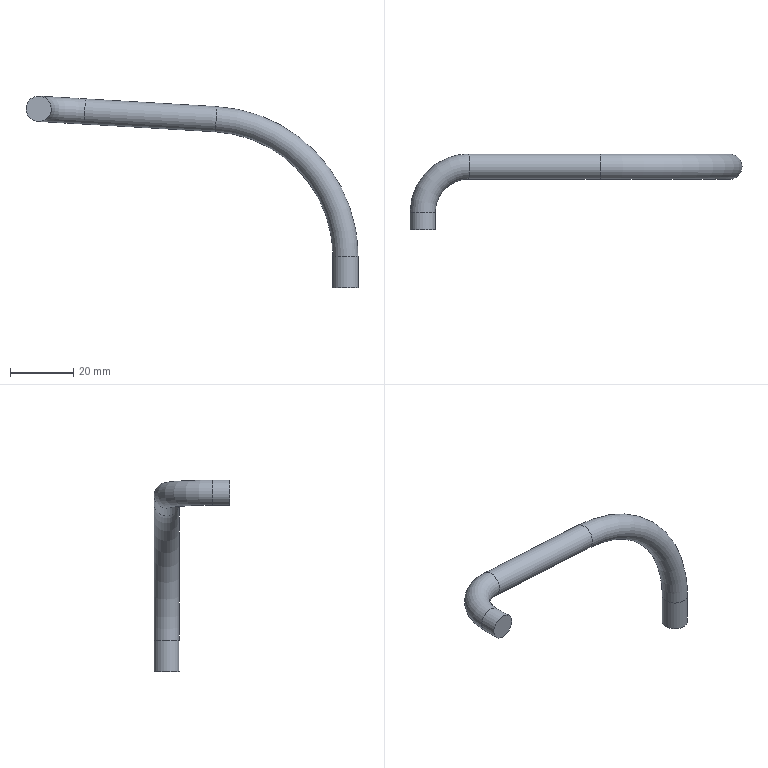Part | STEP file | DEWALT-DWE7294-B3-02 | 1 solid | 7 faces | box 105.161 x 24.081 x 60.688 mm | volume 7333 mm3 | cylinder 3 | torus 2 | plane 2 | commonest cylinder face diameters 8 x3
STEP:
#1=CARTESIAN_POINT('',(0.,0.,0.));
#2=DIRECTION('',(0.,0.,1.));
#3=DIRECTION('',(1.,0.,0.));
#4=AXIS2_PLACEMENT_3D('',#1,#2,#3);
#5=CARTESIAN_POINT('',(4.,0.,0.));
#6=VERTEX_POINT('',#5);
#7=CARTESIAN_POINT('',(0.,0.,0.));
#8=DIRECTION('',(0.,0.,-1.));
#9=DIRECTION('',(1.,0.,0.));
#10=AXIS2_PLACEMENT_3D('',#7,#8,#9);
#11=CIRCLE('',#10,4.);
#12=CARTESIAN_POINT('',(0.,0.,10.));
#13=DIRECTION('',(0.,0.,-1.));
#14=DIRECTION('',(-1.,0.,0.));
#15=AXIS2_PLACEMENT_3D('',#12,#13,#14);
#16=CYLINDRICAL_SURFACE('',#15,4.);
#17=CARTESIAN_POINT('',(3.142,10.));
#18=DIRECTION('',(1.,0.));
#19=VECTOR('',#18,1.);
#20=LINE('',#17,#19);
#21=(GEOMETRIC_REPRESENTATION_CONTEXT(2)PARAMETRIC_REPRESENTATION_CONTEXT()REPRESENTATION_CONTEXT('',''));
#22=DEFINITIONAL_REPRESENTATION('',(#20),#21);
#23=PCURVE('',#16,#22);
#24=CARTESIAN_POINT('',(0.,0.,0.));
#25=DIRECTION('',(0.,0.,-1.));
#26=DIRECTION('',(-1.,0.,0.));
#27=AXIS2_PLACEMENT_3D('',#24,#25,#26);
#28=PLANE('',#27);
#29=CARTESIAN_POINT('',(0.,0.));
#30=DIRECTION('',(-1.,0.));
#31=AXIS2_PLACEMENT_2D('',#29,#30);
#32=CIRCLE('',#31,4.);
#33=(GEOMETRIC_REPRESENTATION_CONTEXT(2)PARAMETRIC_REPRESENTATION_CONTEXT()REPRESENTATION_CONTEXT('',''));
#34=DEFINITIONAL_REPRESENTATION('',(#32),#33);
#35=PCURVE('',#28,#34);
#36=SURFACE_CURVE('',#11,(#23,#35),.PCURVE_S1.);
#37=EDGE_CURVE('',#6,#6,#36,.T.);
#38=ORIENTED_EDGE('',*,*,#37,.F.);
#39=CARTESIAN_POINT('',(4.,0.,10.));
#40=VERTEX_POINT('',#39);
#41=CARTESIAN_POINT('',(4.,0.,10.));
#42=CARTESIAN_POINT('',(4.,0.,0.));
#43=B_SPLINE_CURVE_WITH_KNOTS('',1,(#41,#42),.UNSPECIFIED.,.F.,.F.,(2,2),(0.,10.),.PIECEWISE_BEZIER_KNOTS.);
#44=CARTESIAN_POINT('',(3.142,0.));
#45=DIRECTION('',(0.,1.));
#46=VECTOR('',#45,1.);
#47=LINE('',#44,#46);
#48=(GEOMETRIC_REPRESENTATION_CONTEXT(2)PARAMETRIC_REPRESENTATION_CONTEXT()REPRESENTATION_CONTEXT('',''));
#49=DEFINITIONAL_REPRESENTATION('',(#47),#48);
#50=PCURVE('',#16,#49);
#51=CARTESIAN_POINT('',(9.425,0.));
#52=DIRECTION('',(0.,1.));
#53=VECTOR('',#52,1.);
#54=LINE('',#51,#53);
#55=(GEOMETRIC_REPRESENTATION_CONTEXT(2)PARAMETRIC_REPRESENTATION_CONTEXT()REPRESENTATION_CONTEXT('',''));
#56=DEFINITIONAL_REPRESENTATION('',(#54),#55);
#57=PCURVE('',#16,#56);
#58=SEAM_CURVE('',#43,(#50,#57),.PCURVE_S1.);
#59=EDGE_CURVE('',#40,#6,#58,.T.);
#60=ORIENTED_EDGE('',*,*,#59,.F.);
#61=CARTESIAN_POINT('',(0.,0.,10.));
#62=DIRECTION('',(0.,0.,-1.));
#63=DIRECTION('',(1.,0.,0.));
#64=AXIS2_PLACEMENT_3D('',#61,#62,#63);
#65=CIRCLE('',#64,4.);
#66=CARTESIAN_POINT('',(3.142,0.));
#67=DIRECTION('',(1.,0.));
#68=VECTOR('',#67,1.);
#69=LINE('',#66,#68);
#70=(GEOMETRIC_REPRESENTATION_CONTEXT(2)PARAMETRIC_REPRESENTATION_CONTEXT()REPRESENTATION_CONTEXT('',''));
#71=DEFINITIONAL_REPRESENTATION('',(#69),#70);
#72=PCURVE('',#16,#71);
#73=CARTESIAN_POINT('',(-43.471,0.,10.));
#74=DIRECTION('',(0.,1.,0.));
#75=DIRECTION('',(-1.,0.,0.));
#76=AXIS2_PLACEMENT_3D('',#73,#74,#75);
#77=TOROIDAL_SURFACE('',#76,43.471,4.);
#78=CARTESIAN_POINT('',(3.142,6.283));
#79=DIRECTION('',(0.,-1.));
#80=VECTOR('',#79,1.);
#81=LINE('',#78,#80);
#82=(GEOMETRIC_REPRESENTATION_CONTEXT(2)PARAMETRIC_REPRESENTATION_CONTEXT()REPRESENTATION_CONTEXT('',''));
#83=DEFINITIONAL_REPRESENTATION('',(#81),#82);
#84=PCURVE('',#77,#83);
#85=SURFACE_CURVE('',#65,(#72,#84),.PCURVE_S1.);
#86=EDGE_CURVE('',#40,#40,#85,.T.);
#87=ORIENTED_EDGE('',*,*,#86,.T.);
#88=ORIENTED_EDGE('',*,*,#59,.T.);
#89=EDGE_LOOP('',(#38,#60,#87,#88));
#90=FACE_BOUND('',#89,.T.);
#91=ADVANCED_FACE('',(#90),#16,.T.);
#92=ORIENTED_EDGE('',*,*,#86,.F.);
#93=CARTESIAN_POINT('',(-40.697,0.,57.39));
#94=VERTEX_POINT('',#93);
#95=CARTESIAN_POINT('',(-40.697,0.,57.39));
#96=CARTESIAN_POINT('',(-28.519,0.,56.677));
#97=CARTESIAN_POINT('',(-16.851,0.,52.256));
#98=CARTESIAN_POINT('',(-6.913,0.,44.481));
#99=CARTESIAN_POINT('',(0.2685,0.,34.106));
#100=CARTESIAN_POINT('',(4.,0.,22.199));
#101=CARTESIAN_POINT('',(4.,0.,10.));
#102=(BOUNDED_CURVE()B_SPLINE_CURVE(6,(#95,#96,#97,#98,#99,#100,#101),.UNSPECIFIED.,.F.,.F.)B_SPLINE_CURVE_WITH_KNOTS((7,7),(1.629,3.142),.PIECEWISE_BEZIER_KNOTS.)CURVE()GEOMETRIC_REPRESENTATION_ITEM()RATIONAL_B_SPLINE_CURVE((1.029,1.009,0.9981,0.9944,0.9981,1.009,1.029))REPRESENTATION_ITEM(''));
#103=CARTESIAN_POINT('',(0.,6.283));
#104=DIRECTION('',(1.,0.));
#105=VECTOR('',#104,1.);
#106=LINE('',#103,#105);
#107=(GEOMETRIC_REPRESENTATION_CONTEXT(2)PARAMETRIC_REPRESENTATION_CONTEXT()REPRESENTATION_CONTEXT('',''));
#108=DEFINITIONAL_REPRESENTATION('',(#106),#107);
#109=PCURVE('',#77,#108);
#110=CARTESIAN_POINT('',(0.,0.));
#111=DIRECTION('',(1.,0.));
#112=VECTOR('',#111,1.);
#113=LINE('',#110,#112);
#114=(GEOMETRIC_REPRESENTATION_CONTEXT(2)PARAMETRIC_REPRESENTATION_CONTEXT()REPRESENTATION_CONTEXT('',''));
#115=DEFINITIONAL_REPRESENTATION('',(#113),#114);
#116=PCURVE('',#77,#115);
#117=SEAM_CURVE('',#102,(#109,#116),.PCURVE_S1.);
#118=EDGE_CURVE('',#94,#40,#117,.T.);
#119=ORIENTED_EDGE('',*,*,#118,.F.);
#120=CARTESIAN_POINT('',(-40.931,0.,53.397));
#121=DIRECTION('',(0.9983,0.,-0.05843));
#122=DIRECTION('',(0.05843,0.,0.9983));
#123=AXIS2_PLACEMENT_3D('',#120,#121,#122);
#124=CIRCLE('',#123,4.);
#125=CARTESIAN_POINT('',(1.629,6.283));
#126=DIRECTION('',(0.,-1.));
#127=VECTOR('',#126,1.);
#128=LINE('',#125,#127);
#129=(GEOMETRIC_REPRESENTATION_CONTEXT(2)PARAMETRIC_REPRESENTATION_CONTEXT()REPRESENTATION_CONTEXT('',''));
#130=DEFINITIONAL_REPRESENTATION('',(#128),#129);
#131=PCURVE('',#77,#130);
#132=CARTESIAN_POINT('',(-82.567,0.,55.834));
#133=DIRECTION('',(0.9983,0.,-0.05843));
#134=DIRECTION('',(-0.05843,0.,-0.9983));
#135=AXIS2_PLACEMENT_3D('',#132,#133,#134);
#136=CYLINDRICAL_SURFACE('',#135,4.);
#137=CARTESIAN_POINT('',(3.142,41.707));
#138=DIRECTION('',(1.,0.));
#139=VECTOR('',#138,1.);
#140=LINE('',#137,#139);
#141=(GEOMETRIC_REPRESENTATION_CONTEXT(2)PARAMETRIC_REPRESENTATION_CONTEXT()REPRESENTATION_CONTEXT('',''));
#142=DEFINITIONAL_REPRESENTATION('',(#140),#141);
#143=PCURVE('',#136,#142);
#144=SURFACE_CURVE('',#124,(#131,#143),.PCURVE_S1.);
#145=EDGE_CURVE('',#94,#94,#144,.T.);
#146=ORIENTED_EDGE('',*,*,#145,.T.);
#147=ORIENTED_EDGE('',*,*,#118,.T.);
#148=EDGE_LOOP('',(#92,#119,#146,#147));
#149=FACE_BOUND('',#148,.T.);
#150=ADVANCED_FACE('',(#149),#77,.T.);
#151=ORIENTED_EDGE('',*,*,#145,.F.);
#152=CARTESIAN_POINT('',(-82.333,0.,59.827));
#153=VERTEX_POINT('',#152);
#154=CARTESIAN_POINT('',(-82.333,0.,59.827));
#155=CARTESIAN_POINT('',(-40.697,0.,57.39));
#156=B_SPLINE_CURVE_WITH_KNOTS('',1,(#154,#155),.UNSPECIFIED.,.F.,.F.,(2,2),(0.,41.707),.PIECEWISE_BEZIER_KNOTS.);
#157=CARTESIAN_POINT('',(3.142,0.));
#158=DIRECTION('',(0.,1.));
#159=VECTOR('',#158,1.);
#160=LINE('',#157,#159);
#161=(GEOMETRIC_REPRESENTATION_CONTEXT(2)PARAMETRIC_REPRESENTATION_CONTEXT()REPRESENTATION_CONTEXT('',''));
#162=DEFINITIONAL_REPRESENTATION('',(#160),#161);
#163=PCURVE('',#136,#162);
#164=CARTESIAN_POINT('',(9.425,0.));
#165=DIRECTION('',(0.,1.));
#166=VECTOR('',#165,1.);
#167=LINE('',#164,#166);
#168=(GEOMETRIC_REPRESENTATION_CONTEXT(2)PARAMETRIC_REPRESENTATION_CONTEXT()REPRESENTATION_CONTEXT('',''));
#169=DEFINITIONAL_REPRESENTATION('',(#167),#168);
#170=PCURVE('',#136,#169);
#171=SEAM_CURVE('',#156,(#163,#170),.PCURVE_S1.);
#172=EDGE_CURVE('',#153,#94,#171,.T.);
#173=ORIENTED_EDGE('',*,*,#172,.F.);
#174=CARTESIAN_POINT('',(-82.567,0.,55.834));
#175=DIRECTION('',(0.9983,0.,-0.05843));
#176=DIRECTION('',(0.05843,0.,0.9983));
#177=AXIS2_PLACEMENT_3D('',#174,#175,#176);
#178=CIRCLE('',#177,4.);
#179=CARTESIAN_POINT('',(3.142,0.));
#180=DIRECTION('',(1.,0.));
#181=VECTOR('',#180,1.);
#182=LINE('',#179,#181);
#183=(GEOMETRIC_REPRESENTATION_CONTEXT(2)PARAMETRIC_REPRESENTATION_CONTEXT()REPRESENTATION_CONTEXT('',''));
#184=DEFINITIONAL_REPRESENTATION('',(#182),#183);
#185=PCURVE('',#136,#184);
#186=CARTESIAN_POINT('',(-82.567,-14.62,55.834));
#187=DIRECTION('',(-0.05843,0.,-0.9983));
#188=DIRECTION('',(-0.9983,0.,0.05843));
#189=AXIS2_PLACEMENT_3D('',#186,#187,#188);
#190=TOROIDAL_SURFACE('',#189,14.62,4.);
#191=CARTESIAN_POINT('',(1.571,4.712));
#192=DIRECTION('',(0.,-1.));
#193=VECTOR('',#192,1.);
#194=LINE('',#191,#193);
#195=(GEOMETRIC_REPRESENTATION_CONTEXT(2)PARAMETRIC_REPRESENTATION_CONTEXT()REPRESENTATION_CONTEXT('',''));
#196=DEFINITIONAL_REPRESENTATION('',(#194),#195);
#197=PCURVE('',#190,#196);
#198=SURFACE_CURVE('',#178,(#185,#197),.PCURVE_S1.);
#199=EDGE_CURVE('',#153,#153,#198,.T.);
#200=ORIENTED_EDGE('',*,*,#199,.T.);
#201=ORIENTED_EDGE('',*,*,#172,.T.);
#202=EDGE_LOOP('',(#151,#173,#200,#201));
#203=FACE_BOUND('',#202,.T.);
#204=ADVANCED_FACE('',(#203),#136,.T.);
#205=ORIENTED_EDGE('',*,*,#199,.F.);
#206=CARTESIAN_POINT('',(-96.928,-14.62,60.681));
#207=VERTEX_POINT('',#206);
#208=CARTESIAN_POINT('',(-96.928,-14.62,60.681));
#209=CARTESIAN_POINT('',(-96.928,-10.711,60.681));
#210=CARTESIAN_POINT('',(-95.687,-6.905,60.608));
#211=CARTESIAN_POINT('',(-93.307,-3.627,60.469));
#212=CARTESIAN_POINT('',(-90.035,-1.243,60.278));
#213=CARTESIAN_POINT('',(-86.235,0.,60.055));
#214=CARTESIAN_POINT('',(-82.333,0.,59.827));
#215=(BOUNDED_CURVE()B_SPLINE_CURVE(6,(#208,#209,#210,#211,#212,#213,#214),.UNSPECIFIED.,.F.,.F.)B_SPLINE_CURVE_WITH_KNOTS((7,7),(0.,1.571),.PIECEWISE_BEZIER_KNOTS.)CURVE()GEOMETRIC_REPRESENTATION_ITEM()RATIONAL_B_SPLINE_CURVE((1.031,1.01,0.9979,0.994,0.9979,1.01,1.031))REPRESENTATION_ITEM(''));
#216=CARTESIAN_POINT('',(0.,4.712));
#217=DIRECTION('',(1.,0.));
#218=VECTOR('',#217,1.);
#219=LINE('',#216,#218);
#220=(GEOMETRIC_REPRESENTATION_CONTEXT(2)PARAMETRIC_REPRESENTATION_CONTEXT()REPRESENTATION_CONTEXT('',''));
#221=DEFINITIONAL_REPRESENTATION('',(#219),#220);
#222=PCURVE('',#190,#221);
#223=CARTESIAN_POINT('',(0.,-1.571));
#224=DIRECTION('',(1.,0.));
#225=VECTOR('',#224,1.);
#226=LINE('',#223,#225);
#227=(GEOMETRIC_REPRESENTATION_CONTEXT(2)PARAMETRIC_REPRESENTATION_CONTEXT()REPRESENTATION_CONTEXT('',''));
#228=DEFINITIONAL_REPRESENTATION('',(#226),#227);
#229=PCURVE('',#190,#228);
#230=SEAM_CURVE('',#215,(#222,#229),.PCURVE_S1.);
#231=EDGE_CURVE('',#207,#153,#230,.T.);
#232=ORIENTED_EDGE('',*,*,#231,.F.);
#233=CARTESIAN_POINT('',(-97.161,-14.62,56.688));
#234=DIRECTION('',(0.,1.,0.));
#235=DIRECTION('',(0.05843,0.,0.9983));
#236=AXIS2_PLACEMENT_3D('',#233,#234,#235);
#237=CIRCLE('',#236,4.);
#238=CARTESIAN_POINT('',(0.,4.712));
#239=DIRECTION('',(0.,-1.));
#240=VECTOR('',#239,1.);
#241=LINE('',#238,#240);
#242=(GEOMETRIC_REPRESENTATION_CONTEXT(2)PARAMETRIC_REPRESENTATION_CONTEXT()REPRESENTATION_CONTEXT('',''));
#243=DEFINITIONAL_REPRESENTATION('',(#241),#242);
#244=PCURVE('',#190,#243);
#245=CARTESIAN_POINT('',(-97.161,-20.081,56.688));
#246=DIRECTION('',(0.,1.,0.));
#247=DIRECTION('',(0.,0.,1.));
#248=AXIS2_PLACEMENT_3D('',#245,#246,#247);
#249=CYLINDRICAL_SURFACE('',#248,4.);
#250=CARTESIAN_POINT('',(0.05846,5.461));
#251=DIRECTION('',(1.,0.));
#252=VECTOR('',#251,1.);
#253=LINE('',#250,#252);
#254=(GEOMETRIC_REPRESENTATION_CONTEXT(2)PARAMETRIC_REPRESENTATION_CONTEXT()REPRESENTATION_CONTEXT('',''));
#255=DEFINITIONAL_REPRESENTATION('',(#253),#254);
#256=PCURVE('',#249,#255);
#257=SURFACE_CURVE('',#237,(#244,#256),.PCURVE_S1.);
#258=EDGE_CURVE('',#207,#207,#257,.T.);
#259=ORIENTED_EDGE('',*,*,#258,.T.);
#260=ORIENTED_EDGE('',*,*,#231,.T.);
#261=EDGE_LOOP('',(#205,#232,#259,#260));
#262=FACE_BOUND('',#261,.T.);
#263=ADVANCED_FACE('',(#262),#190,.T.);
#264=ORIENTED_EDGE('',*,*,#258,.F.);
#265=CARTESIAN_POINT('',(-96.928,-20.081,60.681));
#266=VERTEX_POINT('',#265);
#267=CARTESIAN_POINT('',(-96.928,-20.081,60.681));
#268=CARTESIAN_POINT('',(-96.928,-14.62,60.681));
#269=B_SPLINE_CURVE_WITH_KNOTS('',1,(#267,#268),.UNSPECIFIED.,.F.,.F.,(2,2),(0.,5.461),.PIECEWISE_BEZIER_KNOTS.);
#270=CARTESIAN_POINT('',(0.05846,0.));
#271=DIRECTION('',(0.,1.));
#272=VECTOR('',#271,1.);
#273=LINE('',#270,#272);
#274=(GEOMETRIC_REPRESENTATION_CONTEXT(2)PARAMETRIC_REPRESENTATION_CONTEXT()REPRESENTATION_CONTEXT('',''));
#275=DEFINITIONAL_REPRESENTATION('',(#273),#274);
#276=PCURVE('',#249,#275);
#277=CARTESIAN_POINT('',(6.342,0.));
#278=DIRECTION('',(0.,1.));
#279=VECTOR('',#278,1.);
#280=LINE('',#277,#279);
#281=(GEOMETRIC_REPRESENTATION_CONTEXT(2)PARAMETRIC_REPRESENTATION_CONTEXT()REPRESENTATION_CONTEXT('',''));
#282=DEFINITIONAL_REPRESENTATION('',(#280),#281);
#283=PCURVE('',#249,#282);
#284=SEAM_CURVE('',#269,(#276,#283),.PCURVE_S1.);
#285=EDGE_CURVE('',#266,#207,#284,.T.);
#286=ORIENTED_EDGE('',*,*,#285,.F.);
#287=CARTESIAN_POINT('',(-97.161,-20.081,56.688));
#288=DIRECTION('',(0.,1.,0.));
#289=DIRECTION('',(0.05843,0.,0.9983));
#290=AXIS2_PLACEMENT_3D('',#287,#288,#289);
#291=CIRCLE('',#290,4.);
#292=CARTESIAN_POINT('',(0.05846,0.));
#293=DIRECTION('',(1.,0.));
#294=VECTOR('',#293,1.);
#295=LINE('',#292,#294);
#296=(GEOMETRIC_REPRESENTATION_CONTEXT(2)PARAMETRIC_REPRESENTATION_CONTEXT()REPRESENTATION_CONTEXT('',''));
#297=DEFINITIONAL_REPRESENTATION('',(#295),#296);
#298=PCURVE('',#249,#297);
#299=CARTESIAN_POINT('',(-97.161,-20.081,56.688));
#300=DIRECTION('',(0.,1.,0.));
#301=DIRECTION('',(-0.05843,0.,-0.9983));
#302=AXIS2_PLACEMENT_3D('',#299,#300,#301);
#303=PLANE('',#302);
#304=CARTESIAN_POINT('',(0.,0.));
#305=DIRECTION('',(-1.,0.));
#306=AXIS2_PLACEMENT_2D('',#304,#305);
#307=CIRCLE('',#306,4.);
#308=(GEOMETRIC_REPRESENTATION_CONTEXT(2)PARAMETRIC_REPRESENTATION_CONTEXT()REPRESENTATION_CONTEXT('',''));
#309=DEFINITIONAL_REPRESENTATION('',(#307),#308);
#310=PCURVE('',#303,#309);
#311=SURFACE_CURVE('',#291,(#298,#310),.PCURVE_S1.);
#312=EDGE_CURVE('',#266,#266,#311,.T.);
#313=ORIENTED_EDGE('',*,*,#312,.T.);
#314=ORIENTED_EDGE('',*,*,#285,.T.);
#315=EDGE_LOOP('',(#264,#286,#313,#314));
#316=FACE_BOUND('',#315,.T.);
#317=ADVANCED_FACE('',(#316),#249,.T.);
#318=ORIENTED_EDGE('',*,*,#37,.T.);
#319=EDGE_LOOP('',(#318));
#320=FACE_BOUND('',#319,.T.);
#321=ADVANCED_FACE('',(#320),#28,.T.);
#322=ORIENTED_EDGE('',*,*,#312,.F.);
#323=EDGE_LOOP('',(#322));
#324=FACE_BOUND('',#323,.T.);
#325=ADVANCED_FACE('',(#324),#303,.F.);
#326=CLOSED_SHELL('',(#91,#150,#204,#263,#317,#321,#325));
#327=MANIFOLD_SOLID_BREP('',#326);
#328=(LENGTH_UNIT()NAMED_UNIT(*)SI_UNIT(.MILLI.,.METRE.));
#329=UNCERTAINTY_MEASURE_WITH_UNIT(LENGTH_MEASURE(0.000002),#328,'','');
#330=(NAMED_UNIT(*)PLANE_ANGLE_UNIT()SI_UNIT($,.RADIAN.));
#331=(NAMED_UNIT(*)SI_UNIT($,.STERADIAN.)SOLID_ANGLE_UNIT());
#332=(GEOMETRIC_REPRESENTATION_CONTEXT(3)GLOBAL_UNCERTAINTY_ASSIGNED_CONTEXT((#329))GLOBAL_UNIT_ASSIGNED_CONTEXT((#328,#330,#331))REPRESENTATION_CONTEXT('',''));
#333=ADVANCED_BREP_SHAPE_REPRESENTATION('',(#4,#327),#332);